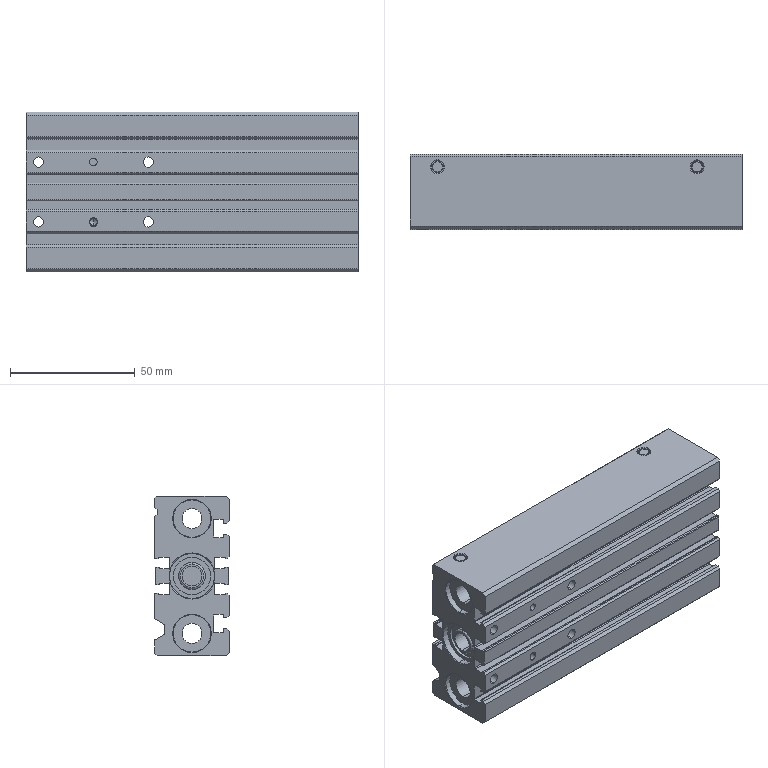Part | STEP file | _TC-L-16x100100_b | 1 solid | 297 faces | box 133 x 30 x 64 mm | volume 175806 mm3 | cylinder 130 | plane 101 | cone 64 | torus 2 | commonest cylinder face diameters 0.8 x20 4.134 x20 0.4 x16 3 x14 8 x14 4.5 x8